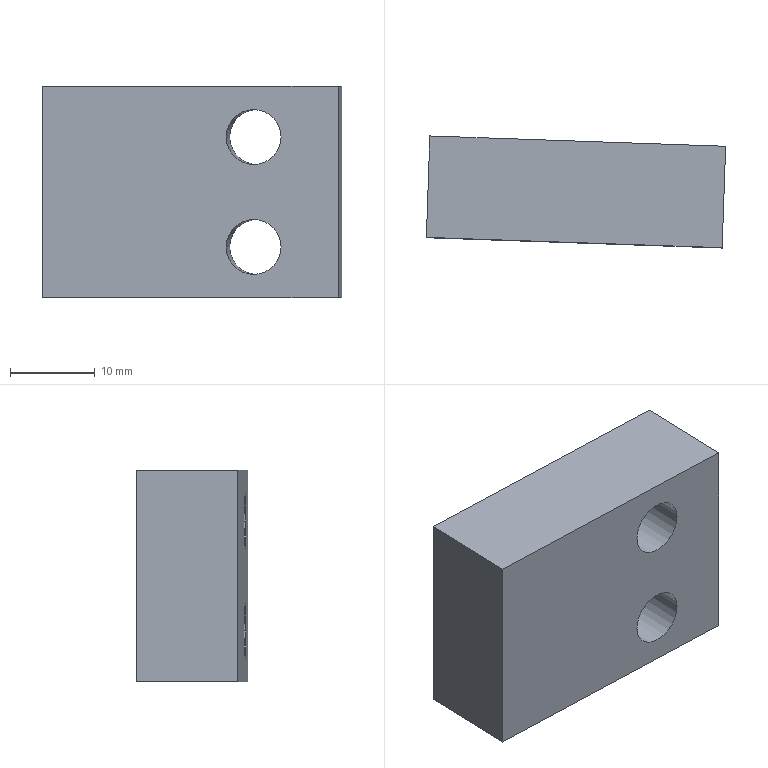Part | STEP file | 1_id1450_x_t | 1 solid | 10 faces | box 35.397 x 13.214 x 25 mm | volume 9704 mm3 | plane 6 | cylinder 4 | commonest cylinder face diameters 6.5 x4
STEP:
#1=CARTESIAN_POINT('',(0.,0.,0.));
#2=DIRECTION('',(0.,0.,1.));
#3=DIRECTION('',(1.,0.,0.));
#4=AXIS2_PLACEMENT_3D('',#1,#2,#3);
#5=CARTESIAN_POINT('',(976.275,186.065,37.96));
#6=VERTEX_POINT('',#5);
#7=CARTESIAN_POINT('',(982.771,185.838,37.96));
#8=VERTEX_POINT('',#7);
#9=CARTESIAN_POINT('',(979.523,185.951,37.96));
#10=DIRECTION('',(-0.0349,-0.9994,0.));
#11=DIRECTION('',(-0.9994,0.0349,0.));
#12=AXIS2_PLACEMENT_3D('',#9,#10,#11);
#13=CIRCLE('',#12,3.25);
#14=CARTESIAN_POINT('',(978.991,170.71,37.96));
#15=DIRECTION('',(-0.0349,-0.9994,0.));
#16=DIRECTION('',(0.9994,-0.0349,0.));
#17=AXIS2_PLACEMENT_3D('',#14,#15,#16);
#18=CYLINDRICAL_SURFACE('',#17,3.25);
#19=CARTESIAN_POINT('',(3.142,-15.25));
#20=DIRECTION('',(1.,0.));
#21=VECTOR('',#20,1.);
#22=LINE('',#19,#21);
#23=(GEOMETRIC_REPRESENTATION_CONTEXT(2)PARAMETRIC_REPRESENTATION_CONTEXT()REPRESENTATION_CONTEXT('',''));
#24=DEFINITIONAL_REPRESENTATION('',(#22),#23);
#25=PCURVE('',#18,#24);
#26=CARTESIAN_POINT('',(944.545,187.173,15.96));
#27=DIRECTION('',(0.0349,0.9994,0.));
#28=DIRECTION('',(0.,0.,-1.));
#29=AXIS2_PLACEMENT_3D('',#26,#27,#28);
#30=PLANE('',#29);
#31=CARTESIAN_POINT('',(-22.,-31.75));
#32=CARTESIAN_POINT('',(-16.371,-31.75));
#33=CARTESIAN_POINT('',(-19.185,-36.625));
#34=CARTESIAN_POINT('',(-22.,-41.5));
#35=CARTESIAN_POINT('',(-24.815,-36.625));
#36=CARTESIAN_POINT('',(-27.629,-31.75));
#37=CARTESIAN_POINT('',(-22.,-31.75));
#38=(BOUNDED_CURVE()B_SPLINE_CURVE(2,(#31,#32,#33,#34,#35,#36,#37),.UNSPECIFIED.,.T.,.F.)B_SPLINE_CURVE_WITH_KNOTS((1,2,2,2,2,1),(-2.094,0.,2.094,4.189,6.283,8.378),.UNSPECIFIED.)CURVE()GEOMETRIC_REPRESENTATION_ITEM()RATIONAL_B_SPLINE_CURVE((1.,0.5,1.,0.5,1.,0.5,1.))REPRESENTATION_ITEM(''));
#39=(GEOMETRIC_REPRESENTATION_CONTEXT(2)PARAMETRIC_REPRESENTATION_CONTEXT()REPRESENTATION_CONTEXT('',''));
#40=DEFINITIONAL_REPRESENTATION('',(#38),#39);
#41=PCURVE('',#30,#40);
#42=SURFACE_CURVE('',#13,(#25,#41),.PCURVE_S1.);
#43=EDGE_CURVE('',#6,#8,#42,.T.);
#44=ORIENTED_EDGE('',*,*,#43,.T.);
#45=CARTESIAN_POINT('',(982.353,173.845,37.96));
#46=VERTEX_POINT('',#45);
#47=CARTESIAN_POINT('',(982.771,185.838,37.96));
#48=DIRECTION('',(-0.0349,-0.9994,0.));
#49=VECTOR('',#48,1.);
#50=LINE('',#47,#49);
#51=CARTESIAN_POINT('',(6.283,-15.25));
#52=DIRECTION('',(0.,1.));
#53=VECTOR('',#52,1.);
#54=LINE('',#51,#53);
#55=(GEOMETRIC_REPRESENTATION_CONTEXT(2)PARAMETRIC_REPRESENTATION_CONTEXT()REPRESENTATION_CONTEXT('',''));
#56=DEFINITIONAL_REPRESENTATION('',(#54),#55);
#57=PCURVE('',#18,#56);
#58=CARTESIAN_POINT('',(978.991,170.71,37.96));
#59=DIRECTION('',(-0.0349,-0.9994,0.));
#60=DIRECTION('',(0.9994,-0.0349,0.));
#61=AXIS2_PLACEMENT_3D('',#58,#59,#60);
#62=CYLINDRICAL_SURFACE('',#61,3.25);
#63=CARTESIAN_POINT('',(0.,-15.25));
#64=DIRECTION('',(0.,1.));
#65=VECTOR('',#64,1.);
#66=LINE('',#63,#65);
#67=(GEOMETRIC_REPRESENTATION_CONTEXT(2)PARAMETRIC_REPRESENTATION_CONTEXT()REPRESENTATION_CONTEXT('',''));
#68=DEFINITIONAL_REPRESENTATION('',(#66),#67);
#69=PCURVE('',#62,#68);
#70=SURFACE_CURVE('',#50,(#57,#69),.PCURVE_S1.);
#71=EDGE_CURVE('',#8,#46,#70,.T.);
#72=ORIENTED_EDGE('',*,*,#71,.T.);
#73=CARTESIAN_POINT('',(975.857,174.072,37.96));
#74=VERTEX_POINT('',#73);
#75=CARTESIAN_POINT('',(979.105,173.959,37.96));
#76=DIRECTION('',(0.0349,0.9994,0.));
#77=DIRECTION('',(0.9994,-0.0349,0.));
#78=AXIS2_PLACEMENT_3D('',#75,#76,#77);
#79=CIRCLE('',#78,3.25);
#80=CARTESIAN_POINT('',(6.283,-3.25));
#81=DIRECTION('',(-1.,0.));
#82=VECTOR('',#81,1.);
#83=LINE('',#80,#82);
#84=(GEOMETRIC_REPRESENTATION_CONTEXT(2)PARAMETRIC_REPRESENTATION_CONTEXT()REPRESENTATION_CONTEXT('',''));
#85=DEFINITIONAL_REPRESENTATION('',(#83),#84);
#86=PCURVE('',#18,#85);
#87=CARTESIAN_POINT('',(998.241,173.29,9.388));
#88=DIRECTION('',(-0.0349,-0.9994,0.));
#89=DIRECTION('',(0.,0.,1.));
#90=AXIS2_PLACEMENT_3D('',#87,#88,#89);
#91=PLANE('',#90);
#92=CARTESIAN_POINT('',(28.572,15.898));
#93=CARTESIAN_POINT('',(22.942,15.898));
#94=CARTESIAN_POINT('',(25.757,20.773));
#95=CARTESIAN_POINT('',(28.572,25.648));
#96=CARTESIAN_POINT('',(31.386,20.773));
#97=CARTESIAN_POINT('',(34.201,15.898));
#98=CARTESIAN_POINT('',(28.572,15.898));
#99=(BOUNDED_CURVE()B_SPLINE_CURVE(2,(#92,#93,#94,#95,#96,#97,#98),.UNSPECIFIED.,.T.,.F.)B_SPLINE_CURVE_WITH_KNOTS((1,2,2,2,2,1),(-2.094,0.,2.094,4.189,6.283,8.378),.UNSPECIFIED.)CURVE()GEOMETRIC_REPRESENTATION_ITEM()RATIONAL_B_SPLINE_CURVE((1.,0.5,1.,0.5,1.,0.5,1.))REPRESENTATION_ITEM(''));
#100=(GEOMETRIC_REPRESENTATION_CONTEXT(2)PARAMETRIC_REPRESENTATION_CONTEXT()REPRESENTATION_CONTEXT('',''));
#101=DEFINITIONAL_REPRESENTATION('',(#99),#100);
#102=PCURVE('',#91,#101);
#103=SURFACE_CURVE('',#79,(#86,#102),.PCURVE_S1.);
#104=EDGE_CURVE('',#46,#74,#103,.T.);
#105=ORIENTED_EDGE('',*,*,#104,.T.);
#106=CARTESIAN_POINT('',(976.275,186.065,37.96));
#107=DIRECTION('',(0.0349,0.9994,0.));
#108=VECTOR('',#107,1.);
#109=LINE('',#106,#108);
#110=CARTESIAN_POINT('',(3.142,-15.25));
#111=DIRECTION('',(0.,-1.));
#112=VECTOR('',#111,1.);
#113=LINE('',#110,#112);
#114=(GEOMETRIC_REPRESENTATION_CONTEXT(2)PARAMETRIC_REPRESENTATION_CONTEXT()REPRESENTATION_CONTEXT('',''));
#115=DEFINITIONAL_REPRESENTATION('',(#113),#114);
#116=PCURVE('',#18,#115);
#117=CARTESIAN_POINT('',(3.142,-15.25));
#118=DIRECTION('',(0.,-1.));
#119=VECTOR('',#118,1.);
#120=LINE('',#117,#119);
#121=(GEOMETRIC_REPRESENTATION_CONTEXT(2)PARAMETRIC_REPRESENTATION_CONTEXT()REPRESENTATION_CONTEXT('',''));
#122=DEFINITIONAL_REPRESENTATION('',(#120),#121);
#123=PCURVE('',#62,#122);
#124=SURFACE_CURVE('',#109,(#116,#123),.PCURVE_S1.);
#125=EDGE_CURVE('',#74,#6,#124,.T.);
#126=ORIENTED_EDGE('',*,*,#125,.T.);
#127=EDGE_LOOP('',(#44,#72,#105,#126));
#128=FACE_BOUND('',#127,.F.);
#129=ADVANCED_FACE('',(#128),#18,.F.);
#130=CARTESIAN_POINT('',(954.539,186.824,18.96));
#131=VERTEX_POINT('',#130);
#132=CARTESIAN_POINT('',(989.517,185.602,18.96));
#133=VERTEX_POINT('',#132);
#134=CARTESIAN_POINT('',(954.539,186.824,18.96));
#135=DIRECTION('',(0.9994,-0.0349,0.));
#136=VECTOR('',#135,1.);
#137=LINE('',#134,#136);
#138=CARTESIAN_POINT('',(-3.,-10.));
#139=DIRECTION('',(0.,-1.));
#140=VECTOR('',#139,1.);
#141=LINE('',#138,#140);
#142=(GEOMETRIC_REPRESENTATION_CONTEXT(2)PARAMETRIC_REPRESENTATION_CONTEXT()REPRESENTATION_CONTEXT('',''));
#143=DEFINITIONAL_REPRESENTATION('',(#141),#142);
#144=PCURVE('',#30,#143);
#145=CARTESIAN_POINT('',(944.31,180.45,18.96));
#146=DIRECTION('',(0.,0.,-1.));
#147=DIRECTION('',(0.,1.,0.));
#148=AXIS2_PLACEMENT_3D('',#145,#146,#147);
#149=PLANE('',#148);
#150=CARTESIAN_POINT('',(6.374,10.229));
#151=DIRECTION('',(-0.0349,0.9994));
#152=VECTOR('',#151,1.);
#153=LINE('',#150,#152);
#154=(GEOMETRIC_REPRESENTATION_CONTEXT(2)PARAMETRIC_REPRESENTATION_CONTEXT()REPRESENTATION_CONTEXT('',''));
#155=DEFINITIONAL_REPRESENTATION('',(#153),#154);
#156=PCURVE('',#149,#155);
#157=SURFACE_CURVE('',#137,(#144,#156),.PCURVE_S1.);
#158=EDGE_CURVE('',#131,#133,#157,.T.);
#159=ORIENTED_EDGE('',*,*,#158,.F.);
#160=CARTESIAN_POINT('',(954.539,186.824,43.96));
#161=VERTEX_POINT('',#160);
#162=CARTESIAN_POINT('',(954.539,186.824,43.96));
#163=DIRECTION('',(0.,0.,-1.));
#164=VECTOR('',#163,1.);
#165=LINE('',#162,#164);
#166=CARTESIAN_POINT('',(-28.,-10.));
#167=DIRECTION('',(1.,0.));
#168=VECTOR('',#167,1.);
#169=LINE('',#166,#168);
#170=(GEOMETRIC_REPRESENTATION_CONTEXT(2)PARAMETRIC_REPRESENTATION_CONTEXT()REPRESENTATION_CONTEXT('',''));
#171=DEFINITIONAL_REPRESENTATION('',(#169),#170);
#172=PCURVE('',#30,#171);
#173=CARTESIAN_POINT('',(954.304,180.101,15.96));
#174=DIRECTION('',(-0.9994,0.0349,0.));
#175=DIRECTION('',(0.,0.,1.));
#176=AXIS2_PLACEMENT_3D('',#173,#174,#175);
#177=PLANE('',#176);
#178=CARTESIAN_POINT('',(28.,6.727));
#179=DIRECTION('',(-1.,0.));
#180=VECTOR('',#179,1.);
#181=LINE('',#178,#180);
#182=(GEOMETRIC_REPRESENTATION_CONTEXT(2)PARAMETRIC_REPRESENTATION_CONTEXT()REPRESENTATION_CONTEXT('',''));
#183=DEFINITIONAL_REPRESENTATION('',(#181),#182);
#184=PCURVE('',#177,#183);
#185=SURFACE_CURVE('',#165,(#172,#184),.PCURVE_S1.);
#186=EDGE_CURVE('',#161,#131,#185,.T.);
#187=ORIENTED_EDGE('',*,*,#186,.F.);
#188=CARTESIAN_POINT('',(989.517,185.602,43.96));
#189=VERTEX_POINT('',#188);
#190=CARTESIAN_POINT('',(989.517,185.602,43.96));
#191=DIRECTION('',(-0.9994,0.0349,0.));
#192=VECTOR('',#191,1.);
#193=LINE('',#190,#192);
#194=CARTESIAN_POINT('',(-28.,-45.));
#195=DIRECTION('',(0.,1.));
#196=VECTOR('',#195,1.);
#197=LINE('',#194,#196);
#198=(GEOMETRIC_REPRESENTATION_CONTEXT(2)PARAMETRIC_REPRESENTATION_CONTEXT()REPRESENTATION_CONTEXT('',''));
#199=DEFINITIONAL_REPRESENTATION('',(#197),#198);
#200=PCURVE('',#30,#199);
#201=CARTESIAN_POINT('',(944.31,180.45,43.96));
#202=DIRECTION('',(0.,0.,1.));
#203=DIRECTION('',(1.,0.,0.));
#204=AXIS2_PLACEMENT_3D('',#201,#202,#203);
#205=PLANE('',#204);
#206=CARTESIAN_POINT('',(45.207,5.153));
#207=DIRECTION('',(-0.9994,0.0349));
#208=VECTOR('',#207,1.);
#209=LINE('',#206,#208);
#210=(GEOMETRIC_REPRESENTATION_CONTEXT(2)PARAMETRIC_REPRESENTATION_CONTEXT()REPRESENTATION_CONTEXT('',''));
#211=DEFINITIONAL_REPRESENTATION('',(#209),#210);
#212=PCURVE('',#205,#211);
#213=SURFACE_CURVE('',#193,(#200,#212),.PCURVE_S1.);
#214=EDGE_CURVE('',#189,#161,#213,.T.);
#215=ORIENTED_EDGE('',*,*,#214,.F.);
#216=CARTESIAN_POINT('',(989.517,185.602,43.96));
#217=DIRECTION('',(0.,0.,-1.));
#218=VECTOR('',#217,1.);
#219=LINE('',#216,#218);
#220=CARTESIAN_POINT('',(-28.,-45.));
#221=DIRECTION('',(1.,0.));
#222=VECTOR('',#221,1.);
#223=LINE('',#220,#222);
#224=(GEOMETRIC_REPRESENTATION_CONTEXT(2)PARAMETRIC_REPRESENTATION_CONTEXT()REPRESENTATION_CONTEXT('',''));
#225=DEFINITIONAL_REPRESENTATION('',(#223),#224);
#226=PCURVE('',#30,#225);
#227=CARTESIAN_POINT('',(989.282,178.879,15.96));
#228=DIRECTION('',(0.9994,-0.0349,0.));
#229=DIRECTION('',(-0.0349,-0.9994,0.));
#230=AXIS2_PLACEMENT_3D('',#227,#228,#229);
#231=PLANE('',#230);
#232=CARTESIAN_POINT('',(-6.727,-28.));
#233=DIRECTION('',(0.,1.));
#234=VECTOR('',#233,1.);
#235=LINE('',#232,#234);
#236=(GEOMETRIC_REPRESENTATION_CONTEXT(2)PARAMETRIC_REPRESENTATION_CONTEXT()REPRESENTATION_CONTEXT('',''));
#237=DEFINITIONAL_REPRESENTATION('',(#235),#236);
#238=PCURVE('',#231,#237);
#239=SURFACE_CURVE('',#219,(#226,#238),.PCURVE_S1.);
#240=EDGE_CURVE('',#189,#133,#239,.T.);
#241=ORIENTED_EDGE('',*,*,#240,.T.);
#242=EDGE_LOOP('',(#159,#187,#215,#241));
#243=FACE_BOUND('',#242,.T.);
#244=CARTESIAN_POINT('',(976.275,186.065,24.96));
#245=VERTEX_POINT('',#244);
#246=CARTESIAN_POINT('',(982.771,185.838,24.96));
#247=VERTEX_POINT('',#246);
#248=CARTESIAN_POINT('',(979.523,185.951,24.96));
#249=DIRECTION('',(-0.0349,-0.9994,0.));
#250=DIRECTION('',(-0.9994,0.0349,0.));
#251=AXIS2_PLACEMENT_3D('',#248,#249,#250);
#252=CIRCLE('',#251,3.25);
#253=CARTESIAN_POINT('',(-9.,-31.75));
#254=CARTESIAN_POINT('',(-3.371,-31.75));
#255=CARTESIAN_POINT('',(-6.185,-36.625));
#256=CARTESIAN_POINT('',(-9.,-41.5));
#257=CARTESIAN_POINT('',(-11.815,-36.625));
#258=CARTESIAN_POINT('',(-14.629,-31.75));
#259=CARTESIAN_POINT('',(-9.,-31.75));
#260=(BOUNDED_CURVE()B_SPLINE_CURVE(2,(#253,#254,#255,#256,#257,#258,#259),.UNSPECIFIED.,.T.,.F.)B_SPLINE_CURVE_WITH_KNOTS((1,2,2,2,2,1),(-2.094,0.,2.094,4.189,6.283,8.378),.UNSPECIFIED.)CURVE()GEOMETRIC_REPRESENTATION_ITEM()RATIONAL_B_SPLINE_CURVE((1.,0.5,1.,0.5,1.,0.5,1.))REPRESENTATION_ITEM(''));
#261=(GEOMETRIC_REPRESENTATION_CONTEXT(2)PARAMETRIC_REPRESENTATION_CONTEXT()REPRESENTATION_CONTEXT('',''));
#262=DEFINITIONAL_REPRESENTATION('',(#260),#261);
#263=PCURVE('',#30,#262);
#264=CARTESIAN_POINT('',(978.991,170.71,24.96));
#265=DIRECTION('',(-0.0349,-0.9994,0.));
#266=DIRECTION('',(-0.9994,0.0349,0.));
#267=AXIS2_PLACEMENT_3D('',#264,#265,#266);
#268=CYLINDRICAL_SURFACE('',#267,3.25);
#269=CARTESIAN_POINT('',(0.,-15.25));
#270=DIRECTION('',(1.,0.));
#271=VECTOR('',#270,1.);
#272=LINE('',#269,#271);
#273=(GEOMETRIC_REPRESENTATION_CONTEXT(2)PARAMETRIC_REPRESENTATION_CONTEXT()REPRESENTATION_CONTEXT('',''));
#274=DEFINITIONAL_REPRESENTATION('',(#272),#273);
#275=PCURVE('',#268,#274);
#276=SURFACE_CURVE('',#252,(#263,#275),.PCURVE_S1.);
#277=EDGE_CURVE('',#245,#247,#276,.T.);
#278=ORIENTED_EDGE('',*,*,#277,.T.);
#279=CARTESIAN_POINT('',(979.523,185.951,24.96));
#280=DIRECTION('',(-0.0349,-0.9994,0.));
#281=DIRECTION('',(0.9994,-0.0349,0.));
#282=AXIS2_PLACEMENT_3D('',#279,#280,#281);
#283=CIRCLE('',#282,3.25);
#284=CARTESIAN_POINT('',(-9.,-38.25));
#285=CARTESIAN_POINT('',(-14.629,-38.25));
#286=CARTESIAN_POINT('',(-11.815,-33.375));
#287=CARTESIAN_POINT('',(-9.,-28.5));
#288=CARTESIAN_POINT('',(-6.185,-33.375));
#289=CARTESIAN_POINT('',(-3.371,-38.25));
#290=CARTESIAN_POINT('',(-9.,-38.25));
#291=(BOUNDED_CURVE()B_SPLINE_CURVE(2,(#284,#285,#286,#287,#288,#289,#290),.UNSPECIFIED.,.T.,.F.)B_SPLINE_CURVE_WITH_KNOTS((1,2,2,2,2,1),(-2.094,0.,2.094,4.189,6.283,8.378),.UNSPECIFIED.)CURVE()GEOMETRIC_REPRESENTATION_ITEM()RATIONAL_B_SPLINE_CURVE((1.,0.5,1.,0.5,1.,0.5,1.))REPRESENTATION_ITEM(''));
#292=(GEOMETRIC_REPRESENTATION_CONTEXT(2)PARAMETRIC_REPRESENTATION_CONTEXT()REPRESENTATION_CONTEXT('',''));
#293=DEFINITIONAL_REPRESENTATION('',(#291),#292);
#294=PCURVE('',#30,#293);
#295=CARTESIAN_POINT('',(978.991,170.71,24.96));
#296=DIRECTION('',(-0.0349,-0.9994,0.));
#297=DIRECTION('',(-0.9994,0.0349,0.));
#298=AXIS2_PLACEMENT_3D('',#295,#296,#297);
#299=CYLINDRICAL_SURFACE('',#298,3.25);
#300=CARTESIAN_POINT('',(3.142,-15.25));
#301=DIRECTION('',(1.,0.));
#302=VECTOR('',#301,1.);
#303=LINE('',#300,#302);
#304=(GEOMETRIC_REPRESENTATION_CONTEXT(2)PARAMETRIC_REPRESENTATION_CONTEXT()REPRESENTATION_CONTEXT('',''));
#305=DEFINITIONAL_REPRESENTATION('',(#303),#304);
#306=PCURVE('',#299,#305);
#307=SURFACE_CURVE('',#283,(#294,#306),.PCURVE_S1.);
#308=EDGE_CURVE('',#247,#245,#307,.T.);
#309=ORIENTED_EDGE('',*,*,#308,.T.);
#310=EDGE_LOOP('',(#278,#309));
#311=FACE_BOUND('',#310,.T.);
#312=CARTESIAN_POINT('',(979.523,185.951,37.96));
#313=DIRECTION('',(-0.0349,-0.9994,0.));
#314=DIRECTION('',(0.9994,-0.0349,0.));
#315=AXIS2_PLACEMENT_3D('',#312,#313,#314);
#316=CIRCLE('',#315,3.25);
#317=CARTESIAN_POINT('',(-22.,-38.25));
#318=CARTESIAN_POINT('',(-27.629,-38.25));
#319=CARTESIAN_POINT('',(-24.815,-33.375));
#320=CARTESIAN_POINT('',(-22.,-28.5));
#321=CARTESIAN_POINT('',(-19.185,-33.375));
#322=CARTESIAN_POINT('',(-16.371,-38.25));
#323=CARTESIAN_POINT('',(-22.,-38.25));
#324=(BOUNDED_CURVE()B_SPLINE_CURVE(2,(#317,#318,#319,#320,#321,#322,#323),.UNSPECIFIED.,.T.,.F.)B_SPLINE_CURVE_WITH_KNOTS((1,2,2,2,2,1),(-2.094,0.,2.094,4.189,6.283,8.378),.UNSPECIFIED.)CURVE()GEOMETRIC_REPRESENTATION_ITEM()RATIONAL_B_SPLINE_CURVE((1.,0.5,1.,0.5,1.,0.5,1.))REPRESENTATION_ITEM(''));
#325=(GEOMETRIC_REPRESENTATION_CONTEXT(2)PARAMETRIC_REPRESENTATION_CONTEXT()REPRESENTATION_CONTEXT('',''));
#326=DEFINITIONAL_REPRESENTATION('',(#324),#325);
#327=PCURVE('',#30,#326);
#328=CARTESIAN_POINT('',(0.,-15.25));
#329=DIRECTION('',(1.,0.));
#330=VECTOR('',#329,1.);
#331=LINE('',#328,#330);
#332=(GEOMETRIC_REPRESENTATION_CONTEXT(2)PARAMETRIC_REPRESENTATION_CONTEXT()REPRESENTATION_CONTEXT('',''));
#333=DEFINITIONAL_REPRESENTATION('',(#331),#332);
#334=PCURVE('',#62,#333);
#335=SURFACE_CURVE('',#316,(#327,#334),.PCURVE_S1.);
#336=EDGE_CURVE('',#8,#6,#335,.T.);
#337=ORIENTED_EDGE('',*,*,#336,.T.);
#338=ORIENTED_EDGE('',*,*,#43,.T.);
#339=EDGE_LOOP('',(#337,#338));
#340=FACE_BOUND('',#339,.T.);
#341=ADVANCED_FACE('',(#243,#311,#340),#30,.T.);
#342=CARTESIAN_POINT('',(989.098,173.61,43.96));
#343=VERTEX_POINT('',#342);
#344=CARTESIAN_POINT('',(989.098,173.61,18.96));
#345=VERTEX_POINT('',#344);
#346=CARTESIAN_POINT('',(989.098,173.61,43.96));
#347=DIRECTION('',(0.,0.,-1.));
#348=VECTOR('',#347,1.);
#349=LINE('',#346,#348);
#350=CARTESIAN_POINT('',(5.273,-28.));
#351=DIRECTION('',(0.,1.));
#352=VECTOR('',#351,1.);
#353=LINE('',#350,#352);
#354=(GEOMETRIC_REPRESENTATION_CONTEXT(2)PARAMETRIC_REPRESENTATION_CONTEXT()REPRESENTATION_CONTEXT('',''));
#355=DEFINITIONAL_REPRESENTATION('',(#353),#354);
#356=PCURVE('',#231,#355);
#357=CARTESIAN_POINT('',(34.572,9.148));
#358=DIRECTION('',(-1.,0.));
#359=VECTOR('',#358,1.);
#360=LINE('',#357,#359);
#361=(GEOMETRIC_REPRESENTATION_CONTEXT(2)PARAMETRIC_REPRESENTATION_CONTEXT()REPRESENTATION_CONTEXT('',''));
#362=DEFINITIONAL_REPRESENTATION('',(#360),#361);
#363=PCURVE('',#91,#362);
#364=SURFACE_CURVE('',#349,(#356,#363),.PCURVE_S1.);
#365=EDGE_CURVE('',#343,#345,#364,.T.);
#366=ORIENTED_EDGE('',*,*,#365,.T.);
#367=CARTESIAN_POINT('',(989.517,185.602,18.96));
#368=DIRECTION('',(-0.0349,-0.9994,0.));
#369=VECTOR('',#368,1.);
#370=LINE('',#367,#369);
#371=CARTESIAN_POINT('',(-6.727,-3.));
#372=DIRECTION('',(1.,0.));
#373=VECTOR('',#372,1.);
#374=LINE('',#371,#373);
#375=(GEOMETRIC_REPRESENTATION_CONTEXT(2)PARAMETRIC_REPRESENTATION_CONTEXT()REPRESENTATION_CONTEXT('',''));
#376=DEFINITIONAL_REPRESENTATION('',(#374),#375);
#377=PCURVE('',#231,#376);
#378=CARTESIAN_POINT('',(5.153,45.207));
#379=DIRECTION('',(-0.9994,-0.0349));
#380=VECTOR('',#379,1.);
#381=LINE('',#378,#380);
#382=(GEOMETRIC_REPRESENTATION_CONTEXT(2)PARAMETRIC_REPRESENTATION_CONTEXT()REPRESENTATION_CONTEXT('',''));
#383=DEFINITIONAL_REPRESENTATION('',(#381),#382);
#384=PCURVE('',#149,#383);
#385=SURFACE_CURVE('',#370,(#377,#384),.PCURVE_S1.);
#386=EDGE_CURVE('',#133,#345,#385,.T.);
#387=ORIENTED_EDGE('',*,*,#386,.F.);
#388=ORIENTED_EDGE('',*,*,#240,.F.);
#389=CARTESIAN_POINT('',(989.098,173.61,43.96));
#390=DIRECTION('',(0.0349,0.9994,0.));
#391=VECTOR('',#390,1.);
#392=LINE('',#389,#391);
#393=CARTESIAN_POINT('',(5.273,-28.));
#394=DIRECTION('',(-1.,0.));
#395=VECTOR('',#394,1.);
#396=LINE('',#393,#395);
#397=(GEOMETRIC_REPRESENTATION_CONTEXT(2)PARAMETRIC_REPRESENTATION_CONTEXT()REPRESENTATION_CONTEXT('',''));
#398=DEFINITIONAL_REPRESENTATION('',(#396),#397);
#399=PCURVE('',#231,#398);
#400=CARTESIAN_POINT('',(44.789,-6.84));
#401=DIRECTION('',(0.0349,0.9994));
#402=VECTOR('',#401,1.);
#403=LINE('',#400,#402);
#404=(GEOMETRIC_REPRESENTATION_CONTEXT(2)PARAMETRIC_REPRESENTATION_CONTEXT()REPRESENTATION_CONTEXT('',''));
#405=DEFINITIONAL_REPRESENTATION('',(#403),#404);
#406=PCURVE('',#205,#405);
#407=SURFACE_CURVE('',#392,(#399,#406),.PCURVE_S1.);
#408=EDGE_CURVE('',#343,#189,#407,.T.);
#409=ORIENTED_EDGE('',*,*,#408,.F.);
#410=EDGE_LOOP('',(#366,#387,#388,#409));
#411=FACE_BOUND('',#410,.T.);
#412=ADVANCED_FACE('',(#411),#231,.T.);
#413=CARTESIAN_POINT('',(954.12,174.831,43.96));
#414=VERTEX_POINT('',#413);
#415=CARTESIAN_POINT('',(954.12,174.831,43.96));
#416=DIRECTION('',(0.9994,-0.0349,0.));
#417=VECTOR('',#416,1.);
#418=LINE('',#415,#417);
#419=CARTESIAN_POINT('',(9.81,-5.619));
#420=DIRECTION('',(0.9994,-0.0349));
#421=VECTOR('',#420,1.);
#422=LINE('',#419,#421);
#423=(GEOMETRIC_REPRESENTATION_CONTEXT(2)PARAMETRIC_REPRESENTATION_CONTEXT()REPRESENTATION_CONTEXT('',''));
#424=DEFINITIONAL_REPRESENTATION('',(#422),#423);
#425=PCURVE('',#205,#424);
#426=CARTESIAN_POINT('',(34.572,44.148));
#427=DIRECTION('',(0.,-1.));
#428=VECTOR('',#427,1.);
#429=LINE('',#426,#428);
#430=(GEOMETRIC_REPRESENTATION_CONTEXT(2)PARAMETRIC_REPRESENTATION_CONTEXT()REPRESENTATION_CONTEXT('',''));
#431=DEFINITIONAL_REPRESENTATION('',(#429),#430);
#432=PCURVE('',#91,#431);
#433=SURFACE_CURVE('',#418,(#425,#432),.PCURVE_S1.);
#434=EDGE_CURVE('',#414,#343,#433,.T.);
#435=ORIENTED_EDGE('',*,*,#434,.T.);
#436=ORIENTED_EDGE('',*,*,#408,.T.);
#437=ORIENTED_EDGE('',*,*,#214,.T.);
#438=CARTESIAN_POINT('',(954.539,186.824,43.96));
#439=DIRECTION('',(-0.0349,-0.9994,0.));
#440=VECTOR('',#439,1.);
#441=LINE('',#438,#440);
#442=CARTESIAN_POINT('',(10.229,6.374));
#443=DIRECTION('',(-0.0349,-0.9994));
#444=VECTOR('',#443,1.);
#445=LINE('',#442,#444);
#446=(GEOMETRIC_REPRESENTATION_CONTEXT(2)PARAMETRIC_REPRESENTATION_CONTEXT()REPRESENTATION_CONTEXT('',''));
#447=DEFINITIONAL_REPRESENTATION('',(#445),#446);
#448=PCURVE('',#205,#447);
#449=CARTESIAN_POINT('',(28.,6.727));
#450=DIRECTION('',(0.,-1.));
#451=VECTOR('',#450,1.);
#452=LINE('',#449,#451);
#453=(GEOMETRIC_REPRESENTATION_CONTEXT(2)PARAMETRIC_REPRESENTATION_CONTEXT()REPRESENTATION_CONTEXT('',''));
#454=DEFINITIONAL_REPRESENTATION('',(#452),#453);
#455=PCURVE('',#177,#454);
#456=SURFACE_CURVE('',#441,(#448,#455),.PCURVE_S1.);
#457=EDGE_CURVE('',#161,#414,#456,.T.);
#458=ORIENTED_EDGE('',*,*,#457,.T.);
#459=EDGE_LOOP('',(#435,#436,#437,#458));
#460=FACE_BOUND('',#459,.T.);
#461=ADVANCED_FACE('',(#460),#205,.T.);
#462=CARTESIAN_POINT('',(954.12,174.831,18.96));
#463=VERTEX_POINT('',#462);
#464=CARTESIAN_POINT('',(954.12,174.831,18.96));
#465=DIRECTION('',(0.,0.,1.));
#466=VECTOR('',#465,1.);
#467=LINE('',#464,#466);
#468=CARTESIAN_POINT('',(3.,-5.273));
#469=DIRECTION('',(1.,0.));
#470=VECTOR('',#469,1.);
#471=LINE('',#468,#470);
#472=(GEOMETRIC_REPRESENTATION_CONTEXT(2)PARAMETRIC_REPRESENTATION_CONTEXT()REPRESENTATION_CONTEXT('',''));
#473=DEFINITIONAL_REPRESENTATION('',(#471),#472);
#474=PCURVE('',#177,#473);
#475=CARTESIAN_POINT('',(9.572,44.148));
#476=DIRECTION('',(1.,0.));
#477=VECTOR('',#476,1.);
#478=LINE('',#475,#477);
#479=(GEOMETRIC_REPRESENTATION_CONTEXT(2)PARAMETRIC_REPRESENTATION_CONTEXT()REPRESENTATION_CONTEXT('',''));
#480=DEFINITIONAL_REPRESENTATION('',(#478),#479);
#481=PCURVE('',#91,#480);
#482=SURFACE_CURVE('',#467,(#474,#481),.PCURVE_S1.);
#483=EDGE_CURVE('',#463,#414,#482,.T.);
#484=ORIENTED_EDGE('',*,*,#483,.T.);
#485=ORIENTED_EDGE('',*,*,#457,.F.);
#486=ORIENTED_EDGE('',*,*,#186,.T.);
#487=CARTESIAN_POINT('',(954.12,174.831,18.96));
#488=DIRECTION('',(0.0349,0.9994,0.));
#489=VECTOR('',#488,1.);
#490=LINE('',#487,#489);
#491=CARTESIAN_POINT('',(3.,-5.273));
#492=DIRECTION('',(0.,1.));
#493=VECTOR('',#492,1.);
#494=LINE('',#491,#493);
#495=(GEOMETRIC_REPRESENTATION_CONTEXT(2)PARAMETRIC_REPRESENTATION_CONTEXT()REPRESENTATION_CONTEXT('',''));
#496=DEFINITIONAL_REPRESENTATION('',(#494),#495);
#497=PCURVE('',#177,#496);
#498=CARTESIAN_POINT('',(-5.619,9.81));
#499=DIRECTION('',(0.9994,0.0349));
#500=VECTOR('',#499,1.);
#501=LINE('',#498,#500);
#502=(GEOMETRIC_REPRESENTATION_CONTEXT(2)PARAMETRIC_REPRESENTATION_CONTEXT()REPRESENTATION_CONTEXT('',''));
#503=DEFINITIONAL_REPRESENTATION('',(#501),#502);
#504=PCURVE('',#149,#503);
#505=SURFACE_CURVE('',#490,(#497,#504),.PCURVE_S1.);
#506=EDGE_CURVE('',#463,#131,#505,.T.);
#507=ORIENTED_EDGE('',*,*,#506,.F.);
#508=EDGE_LOOP('',(#484,#485,#486,#507));
#509=FACE_BOUND('',#508,.T.);
#510=ADVANCED_FACE('',(#509),#177,.T.);
#511=CARTESIAN_POINT('',(989.098,173.61,18.96));
#512=DIRECTION('',(-0.9994,0.0349,0.));
#513=VECTOR('',#512,1.);
#514=LINE('',#511,#513);
#515=CARTESIAN_POINT('',(-6.84,44.789));
#516=DIRECTION('',(0.0349,-0.9994));
#517=VECTOR('',#516,1.);
#518=LINE('',#515,#517);
#519=(GEOMETRIC_REPRESENTATION_CONTEXT(2)PARAMETRIC_REPRESENTATION_CONTEXT()REPRESENTATION_CONTEXT('',''));
#520=DEFINITIONAL_REPRESENTATION('',(#518),#519);
#521=PCURVE('',#149,#520);
#522=CARTESIAN_POINT('',(9.572,9.148));
#523=DIRECTION('',(0.,1.));
#524=VECTOR('',#523,1.);
#525=LINE('',#522,#524);
#526=(GEOMETRIC_REPRESENTATION_CONTEXT(2)PARAMETRIC_REPRESENTATION_CONTEXT()REPRESENTATION_CONTEXT('',''));
#527=DEFINITIONAL_REPRESENTATION('',(#525),#526);
#528=PCURVE('',#91,#527);
#529=SURFACE_CURVE('',#514,(#521,#528),.PCURVE_S1.);
#530=EDGE_CURVE('',#345,#463,#529,.T.);
#531=ORIENTED_EDGE('',*,*,#530,.T.);
#532=ORIENTED_EDGE('',*,*,#506,.T.);
#533=ORIENTED_EDGE('',*,*,#158,.T.);
#534=ORIENTED_EDGE('',*,*,#386,.T.);
#535=EDGE_LOOP('',(#531,#532,#533,#534));
#536=FACE_BOUND('',#535,.T.);
#537=ADVANCED_FACE('',(#536),#149,.T.);
#538=ORIENTED_EDGE('',*,*,#483,.F.);
#539=ORIENTED_EDGE('',*,*,#530,.F.);
#540=ORIENTED_EDGE('',*,*,#365,.F.);
#541=ORIENTED_EDGE('',*,*,#434,.F.);
#542=EDGE_LOOP('',(#538,#539,#540,#541));
#543=FACE_BOUND('',#542,.T.);
#544=CARTESIAN_POINT('',(982.353,173.845,24.96));
#545=VERTEX_POINT('',#544);
#546=CARTESIAN_POINT('',(975.857,174.072,24.96));
#547=VERTEX_POINT('',#546);
#548=CARTESIAN_POINT('',(979.105,173.959,24.96));
#549=DIRECTION('',(0.0349,0.9994,0.));
#550=DIRECTION('',(0.9994,-0.0349,0.));
#551=AXIS2_PLACEMENT_3D('',#548,#549,#550);
#552=CIRCLE('',#551,3.25);
#553=CARTESIAN_POINT('',(15.572,15.898));
#554=CARTESIAN_POINT('',(9.942,15.898));
#555=CARTESIAN_POINT('',(12.757,20.773));
#556=CARTESIAN_POINT('',(15.572,25.648));
#557=CARTESIAN_POINT('',(18.386,20.773));
#558=CARTESIAN_POINT('',(21.201,15.898));
#559=CARTESIAN_POINT('',(15.572,15.898));
#560=(BOUNDED_CURVE()B_SPLINE_CURVE(2,(#553,#554,#555,#556,#557,#558,#559),.UNSPECIFIED.,.T.,.F.)B_SPLINE_CURVE_WITH_KNOTS((1,2,2,2,2,1),(-2.094,0.,2.094,4.189,6.283,8.378),.UNSPECIFIED.)CURVE()GEOMETRIC_REPRESENTATION_ITEM()RATIONAL_B_SPLINE_CURVE((1.,0.5,1.,0.5,1.,0.5,1.))REPRESENTATION_ITEM(''));
#561=(GEOMETRIC_REPRESENTATION_CONTEXT(2)PARAMETRIC_REPRESENTATION_CONTEXT()REPRESENTATION_CONTEXT('',''));
#562=DEFINITIONAL_REPRESENTATION('',(#560),#561);
#563=PCURVE('',#91,#562);
#564=CARTESIAN_POINT('',(3.142,-3.25));
#565=DIRECTION('',(-1.,0.));
#566=VECTOR('',#565,1.);
#567=LINE('',#564,#566);
#568=(GEOMETRIC_REPRESENTATION_CONTEXT(2)PARAMETRIC_REPRESENTATION_CONTEXT()REPRESENTATION_CONTEXT('',''));
#569=DEFINITIONAL_REPRESENTATION('',(#567),#568);
#570=PCURVE('',#268,#569);
#571=SURFACE_CURVE('',#552,(#563,#570),.PCURVE_S1.);
#572=EDGE_CURVE('',#545,#547,#571,.T.);
#573=ORIENTED_EDGE('',*,*,#572,.T.);
#574=CARTESIAN_POINT('',(979.105,173.959,24.96));
#575=DIRECTION('',(0.0349,0.9994,0.));
#576=DIRECTION('',(-0.9994,0.0349,0.));
#577=AXIS2_PLACEMENT_3D('',#574,#575,#576);
#578=CIRCLE('',#577,3.25);
#579=CARTESIAN_POINT('',(15.572,22.398));
#580=CARTESIAN_POINT('',(21.201,22.398));
#581=CARTESIAN_POINT('',(18.386,17.523));
#582=CARTESIAN_POINT('',(15.572,12.648));
#583=CARTESIAN_POINT('',(12.757,17.523));
#584=CARTESIAN_POINT('',(9.942,22.398));
#585=CARTESIAN_POINT('',(15.572,22.398));
#586=(BOUNDED_CURVE()B_SPLINE_CURVE(2,(#579,#580,#581,#582,#583,#584,#585),.UNSPECIFIED.,.T.,.F.)B_SPLINE_CURVE_WITH_KNOTS((1,2,2,2,2,1),(-2.094,0.,2.094,4.189,6.283,8.378),.UNSPECIFIED.)CURVE()GEOMETRIC_REPRESENTATION_ITEM()RATIONAL_B_SPLINE_CURVE((1.,0.5,1.,0.5,1.,0.5,1.))REPRESENTATION_ITEM(''));
#587=(GEOMETRIC_REPRESENTATION_CONTEXT(2)PARAMETRIC_REPRESENTATION_CONTEXT()REPRESENTATION_CONTEXT('',''));
#588=DEFINITIONAL_REPRESENTATION('',(#586),#587);
#589=PCURVE('',#91,#588);
#590=CARTESIAN_POINT('',(6.283,-3.25));
#591=DIRECTION('',(-1.,0.));
#592=VECTOR('',#591,1.);
#593=LINE('',#590,#592);
#594=(GEOMETRIC_REPRESENTATION_CONTEXT(2)PARAMETRIC_REPRESENTATION_CONTEXT()REPRESENTATION_CONTEXT('',''));
#595=DEFINITIONAL_REPRESENTATION('',(#593),#594);
#596=PCURVE('',#299,#595);
#597=SURFACE_CURVE('',#578,(#589,#596),.PCURVE_S1.);
#598=EDGE_CURVE('',#547,#545,#597,.T.);
#599=ORIENTED_EDGE('',*,*,#598,.T.);
#600=EDGE_LOOP('',(#573,#599));
#601=FACE_BOUND('',#600,.T.);
#602=ORIENTED_EDGE('',*,*,#104,.T.);
#603=CARTESIAN_POINT('',(979.105,173.959,37.96));
#604=DIRECTION('',(0.0349,0.9994,0.));
#605=DIRECTION('',(-0.9994,0.0349,0.));
#606=AXIS2_PLACEMENT_3D('',#603,#604,#605);
#607=CIRCLE('',#606,3.25);
#608=CARTESIAN_POINT('',(28.572,22.398));
#609=CARTESIAN_POINT('',(34.201,22.398));
#610=CARTESIAN_POINT('',(31.386,17.523));
#611=CARTESIAN_POINT('',(28.572,12.648));
#612=CARTESIAN_POINT('',(25.757,17.523));
#613=CARTESIAN_POINT('',(22.942,22.398));
#614=CARTESIAN_POINT('',(28.572,22.398));
#615=(BOUNDED_CURVE()B_SPLINE_CURVE(2,(#608,#609,#610,#611,#612,#613,#614),.UNSPECIFIED.,.T.,.F.)B_SPLINE_CURVE_WITH_KNOTS((1,2,2,2,2,1),(-2.094,0.,2.094,4.189,6.283,8.378),.UNSPECIFIED.)CURVE()GEOMETRIC_REPRESENTATION_ITEM()RATIONAL_B_SPLINE_CURVE((1.,0.5,1.,0.5,1.,0.5,1.))REPRESENTATION_ITEM(''));
#616=(GEOMETRIC_REPRESENTATION_CONTEXT(2)PARAMETRIC_REPRESENTATION_CONTEXT()REPRESENTATION_CONTEXT('',''));
#617=DEFINITIONAL_REPRESENTATION('',(#615),#616);
#618=PCURVE('',#91,#617);
#619=CARTESIAN_POINT('',(3.142,-3.25));
#620=DIRECTION('',(-1.,0.));
#621=VECTOR('',#620,1.);
#622=LINE('',#619,#621);
#623=(GEOMETRIC_REPRESENTATION_CONTEXT(2)PARAMETRIC_REPRESENTATION_CONTEXT()REPRESENTATION_CONTEXT('',''));
#624=DEFINITIONAL_REPRESENTATION('',(#622),#623);
#625=PCURVE('',#62,#624);
#626=SURFACE_CURVE('',#607,(#618,#625),.PCURVE_S1.);
#627=EDGE_CURVE('',#74,#46,#626,.T.);
#628=ORIENTED_EDGE('',*,*,#627,.T.);
#629=EDGE_LOOP('',(#602,#628));
#630=FACE_BOUND('',#629,.T.);
#631=ADVANCED_FACE('',(#543,#601,#630),#91,.T.);
#632=ORIENTED_EDGE('',*,*,#308,.T.);
#633=CARTESIAN_POINT('',(976.275,186.065,24.96));
#634=DIRECTION('',(0.0349,0.9994,0.));
#635=VECTOR('',#634,1.);
#636=LINE('',#633,#635);
#637=CARTESIAN_POINT('',(6.283,-15.25));
#638=DIRECTION('',(0.,-1.));
#639=VECTOR('',#638,1.);
#640=LINE('',#637,#639);
#641=(GEOMETRIC_REPRESENTATION_CONTEXT(2)PARAMETRIC_REPRESENTATION_CONTEXT()REPRESENTATION_CONTEXT('',''));
#642=DEFINITIONAL_REPRESENTATION('',(#640),#641);
#643=PCURVE('',#299,#642);
#644=CARTESIAN_POINT('',(0.,-15.25));
#645=DIRECTION('',(0.,-1.));
#646=VECTOR('',#645,1.);
#647=LINE('',#644,#646);
#648=(GEOMETRIC_REPRESENTATION_CONTEXT(2)PARAMETRIC_REPRESENTATION_CONTEXT()REPRESENTATION_CONTEXT('',''));
#649=DEFINITIONAL_REPRESENTATION('',(#647),#648);
#650=PCURVE('',#268,#649);
#651=SURFACE_CURVE('',#636,(#643,#650),.PCURVE_S1.);
#652=EDGE_CURVE('',#547,#245,#651,.T.);
#653=ORIENTED_EDGE('',*,*,#652,.F.);
#654=ORIENTED_EDGE('',*,*,#598,.T.);
#655=CARTESIAN_POINT('',(982.771,185.838,24.96));
#656=DIRECTION('',(-0.0349,-0.9994,0.));
#657=VECTOR('',#656,1.);
#658=LINE('',#655,#657);
#659=CARTESIAN_POINT('',(3.142,-15.25));
#660=DIRECTION('',(0.,1.));
#661=VECTOR('',#660,1.);
#662=LINE('',#659,#661);
#663=(GEOMETRIC_REPRESENTATION_CONTEXT(2)PARAMETRIC_REPRESENTATION_CONTEXT()REPRESENTATION_CONTEXT('',''));
#664=DEFINITIONAL_REPRESENTATION('',(#662),#663);
#665=PCURVE('',#299,#664);
#666=CARTESIAN_POINT('',(3.142,-15.25));
#667=DIRECTION('',(0.,1.));
#668=VECTOR('',#667,1.);
#669=LINE('',#666,#668);
#670=(GEOMETRIC_REPRESENTATION_CONTEXT(2)PARAMETRIC_REPRESENTATION_CONTEXT()REPRESENTATION_CONTEXT('',''));
#671=DEFINITIONAL_REPRESENTATION('',(#669),#670);
#672=PCURVE('',#268,#671);
#673=SURFACE_CURVE('',#658,(#665,#672),.PCURVE_S1.);
#674=EDGE_CURVE('',#247,#545,#673,.T.);
#675=ORIENTED_EDGE('',*,*,#674,.F.);
#676=EDGE_LOOP('',(#632,#653,#654,#675));
#677=FACE_BOUND('',#676,.F.);
#678=ADVANCED_FACE('',(#677),#299,.F.);
#679=ORIENTED_EDGE('',*,*,#277,.T.);
#680=ORIENTED_EDGE('',*,*,#674,.T.);
#681=ORIENTED_EDGE('',*,*,#572,.T.);
#682=ORIENTED_EDGE('',*,*,#652,.T.);
#683=EDGE_LOOP('',(#679,#680,#681,#682));
#684=FACE_BOUND('',#683,.F.);
#685=ADVANCED_FACE('',(#684),#268,.F.);
#686=ORIENTED_EDGE('',*,*,#336,.T.);
#687=ORIENTED_EDGE('',*,*,#125,.F.);
#688=ORIENTED_EDGE('',*,*,#627,.T.);
#689=ORIENTED_EDGE('',*,*,#71,.F.);
#690=EDGE_LOOP('',(#686,#687,#688,#689));
#691=FACE_BOUND('',#690,.F.);
#692=ADVANCED_FACE('',(#691),#62,.F.);
#693=CLOSED_SHELL('',(#129,#341,#412,#461,#510,#537,#631,#678,#685,#692));
#694=MANIFOLD_SOLID_BREP('',#693);
#695=(LENGTH_UNIT()NAMED_UNIT(*)SI_UNIT(.MILLI.,.METRE.));
#696=UNCERTAINTY_MEASURE_WITH_UNIT(LENGTH_MEASURE(0.0000001),#695,'','');
#697=(NAMED_UNIT(*)PLANE_ANGLE_UNIT()SI_UNIT($,.RADIAN.));
#698=(NAMED_UNIT(*)SI_UNIT($,.STERADIAN.)SOLID_ANGLE_UNIT());
#699=(GEOMETRIC_REPRESENTATION_CONTEXT(3)GLOBAL_UNCERTAINTY_ASSIGNED_CONTEXT((#696))GLOBAL_UNIT_ASSIGNED_CONTEXT((#695,#697,#698))REPRESENTATION_CONTEXT('',''));
#700=ADVANCED_BREP_SHAPE_REPRESENTATION('',(#4,#694),#699);